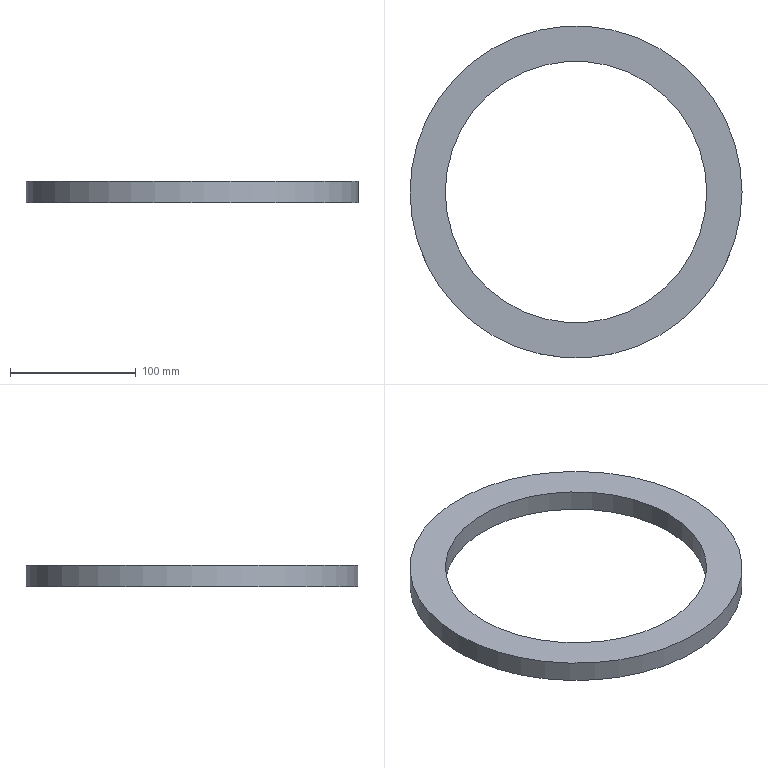Part | NX | features CYLINDER 2, DATUM_CSYS 1, Delete Body 1, LINKED_BODY 1, SCALE 1 | 1 solid | 4 faces | box 264.375 x 264.375 x 16.875 mm | volume 352256 mm3 | plane 2 | cylinder 2 | commonest cylinder face diameters 208.125 x1 264.375 x1
STEP:
#1=CARTESIAN_POINT('',(-470.645,-2029.479,125.625));
#2=VERTEX_POINT('',#1);
#3=CARTESIAN_POINT('',(-366.582,-2029.479,125.625));
#4=DIRECTION('',(0.,0.,-1.));
#5=DIRECTION('',(-1.,0.,0.));
#6=AXIS2_PLACEMENT_3D('',#3,#4,#5);
#7=CIRCLE('',#6,104.062);
#8=EDGE_CURVE('',#2,#2,#7,.T.);
#9=ORIENTED_EDGE('',*,*,#8,.T.);
#10=EDGE_LOOP('',(#9));
#11=FACE_BOUND('',#10,.T.);
#12=CARTESIAN_POINT('',(-498.77,-2029.479,125.625));
#13=VERTEX_POINT('',#12);
#14=CARTESIAN_POINT('',(-366.582,-2029.479,125.625));
#15=DIRECTION('',(0.,0.,-1.));
#16=DIRECTION('',(-1.,0.,0.));
#17=AXIS2_PLACEMENT_3D('',#14,#15,#16);
#18=CIRCLE('',#17,132.188);
#19=EDGE_CURVE('',#13,#13,#18,.T.);
#20=ORIENTED_EDGE('',*,*,#19,.F.);
#21=EDGE_LOOP('',(#20));
#22=FACE_BOUND('',#21,.T.);
#23=CARTESIAN_POINT('',(-366.582,-2029.479,125.625));
#24=DIRECTION('',(0.,0.,1.));
#25=DIRECTION('',(1.,0.,0.));
#26=AXIS2_PLACEMENT_3D('',#23,#24,#25);
#27=PLANE('',#26);
#28=ADVANCED_FACE('',(#11,#22),#27,.T.);
#29=CARTESIAN_POINT('',(-262.52,-2029.479,108.75));
#30=VERTEX_POINT('',#29);
#31=CARTESIAN_POINT('',(-366.582,-2029.479,108.75));
#32=DIRECTION('',(0.,0.,1.));
#33=DIRECTION('',(1.,0.,0.));
#34=AXIS2_PLACEMENT_3D('',#31,#32,#33);
#35=CIRCLE('',#34,104.062);
#36=EDGE_CURVE('',#30,#30,#35,.T.);
#37=ORIENTED_EDGE('',*,*,#36,.T.);
#38=EDGE_LOOP('',(#37));
#39=FACE_BOUND('',#38,.T.);
#40=CARTESIAN_POINT('',(-234.395,-2029.479,108.75));
#41=VERTEX_POINT('',#40);
#42=CARTESIAN_POINT('',(-366.582,-2029.479,108.75));
#43=DIRECTION('',(0.,0.,1.));
#44=DIRECTION('',(1.,0.,0.));
#45=AXIS2_PLACEMENT_3D('',#42,#43,#44);
#46=CIRCLE('',#45,132.188);
#47=EDGE_CURVE('',#41,#41,#46,.T.);
#48=ORIENTED_EDGE('',*,*,#47,.F.);
#49=EDGE_LOOP('',(#48));
#50=FACE_BOUND('',#49,.T.);
#51=CARTESIAN_POINT('',(-366.582,-2029.479,108.75));
#52=DIRECTION('',(0.,0.,-1.));
#53=DIRECTION('',(-1.,0.,0.));
#54=AXIS2_PLACEMENT_3D('',#51,#52,#53);
#55=PLANE('',#54);
#56=ADVANCED_FACE('',(#39,#50),#55,.T.);
#57=ORIENTED_EDGE('',*,*,#19,.T.);
#58=EDGE_LOOP('',(#57));
#59=FACE_BOUND('',#58,.T.);
#60=ORIENTED_EDGE('',*,*,#47,.T.);
#61=EDGE_LOOP('',(#60));
#62=FACE_BOUND('',#61,.T.);
#63=CARTESIAN_POINT('',(-366.582,-2029.479,108.75));
#64=DIRECTION('',(0.,0.,1.));
#65=DIRECTION('',(1.,0.,0.));
#66=AXIS2_PLACEMENT_3D('',#63,#64,#65);
#67=CYLINDRICAL_SURFACE('',#66,132.188);
#68=ADVANCED_FACE('',(#59,#62),#67,.T.);
#69=ORIENTED_EDGE('',*,*,#8,.F.);
#70=EDGE_LOOP('',(#69));
#71=FACE_BOUND('',#70,.T.);
#72=ORIENTED_EDGE('',*,*,#36,.F.);
#73=EDGE_LOOP('',(#72));
#74=FACE_BOUND('',#73,.T.);
#75=CARTESIAN_POINT('',(-366.582,-2029.479,108.75));
#76=DIRECTION('',(0.,0.,1.));
#77=DIRECTION('',(1.,0.,0.));
#78=AXIS2_PLACEMENT_3D('',#75,#76,#77);
#79=CYLINDRICAL_SURFACE('',#78,104.062);
#80=ADVANCED_FACE('',(#71,#74),#79,.F.);
#81=CLOSED_SHELL('',(#28,#56,#68,#80));
#82=MANIFOLD_SOLID_BREP('',#81);
#83=(LENGTH_UNIT()NAMED_UNIT(*)SI_UNIT(.MILLI.,.METRE.));
#84=UNCERTAINTY_MEASURE_WITH_UNIT(LENGTH_MEASURE(0.00001),#83,'','');
#85=(NAMED_UNIT(*)PLANE_ANGLE_UNIT()SI_UNIT($,.RADIAN.));
#86=(NAMED_UNIT(*)SI_UNIT($,.STERADIAN.)SOLID_ANGLE_UNIT());
#87=(GEOMETRIC_REPRESENTATION_CONTEXT(3)GLOBAL_UNCERTAINTY_ASSIGNED_CONTEXT((#84))GLOBAL_UNIT_ASSIGNED_CONTEXT((#83,#85,#86))REPRESENTATION_CONTEXT('',''));
#88=ADVANCED_BREP_SHAPE_REPRESENTATION('',(#82),#87);